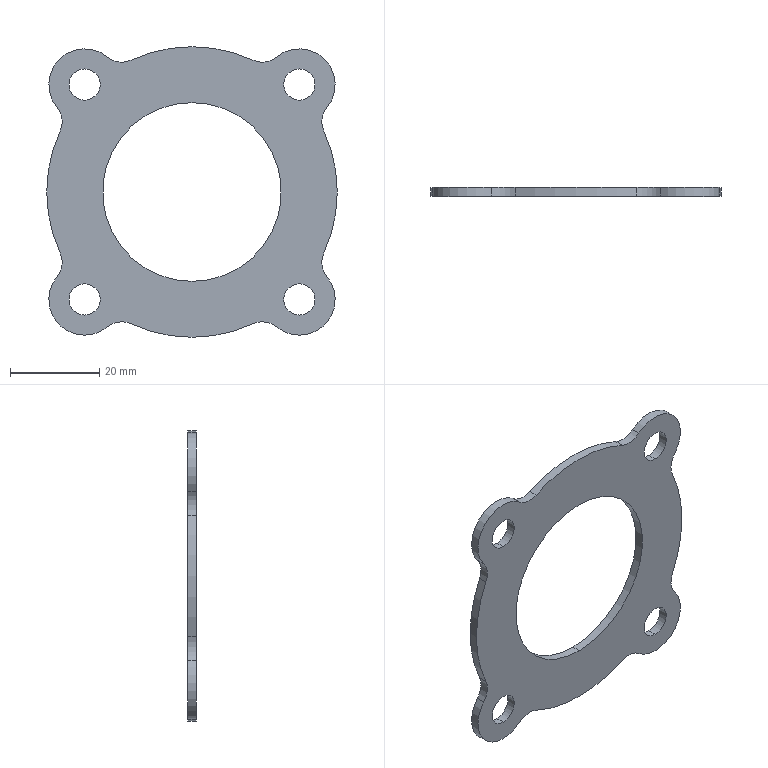Part | SolidWorks | features Fillet 2, Extrusion 1 | 1 solid | 33 faces | box 65 x 2 x 65 mm | volume 4890 mm3 | cylinder 31 | plane 2 | commonest cylinder face diameters 10 x10 7 x8 16 x6 65 x5 40 x2
STEP:
#1=CARTESIAN_POINT('',(-15.733,0.,-29.04));
#2=VERTEX_POINT('',#1);
#3=CARTESIAN_POINT('',(-13.635,0.,-29.501));
#4=VERTEX_POINT('',#3);
#5=CARTESIAN_POINT('',(-15.733,0.,-34.04));
#6=DIRECTION('',(0.,1.,0.));
#7=DIRECTION('',(0.,0.,1.));
#8=AXIS2_PLACEMENT_3D('',#5,#6,#7);
#9=CIRCLE('',#8,5.);
#10=EDGE_CURVE('',#2,#4,#9,.T.);
#11=ORIENTED_EDGE('',*,*,#10,.F.);
#12=CARTESIAN_POINT('',(-15.733,2.,-29.04));
#13=VERTEX_POINT('',#12);
#14=CARTESIAN_POINT('',(-15.733,2.,-29.04));
#15=DIRECTION('',(0.,1.,0.));
#16=VECTOR('',#15,1000.);
#17=LINE('',#14,#16);
#18=EDGE_CURVE('',#2,#13,#17,.T.);
#19=ORIENTED_EDGE('',*,*,#18,.T.);
#20=CARTESIAN_POINT('',(-13.635,2.,-29.501));
#21=VERTEX_POINT('',#20);
#22=CARTESIAN_POINT('',(-15.733,2.,-34.04));
#23=DIRECTION('',(0.,-1.,0.));
#24=DIRECTION('',(0.,0.,1.));
#25=AXIS2_PLACEMENT_3D('',#22,#23,#24);
#26=CIRCLE('',#25,5.);
#27=EDGE_CURVE('',#21,#13,#26,.T.);
#28=ORIENTED_EDGE('',*,*,#27,.F.);
#29=CARTESIAN_POINT('',(-13.635,2.,-29.501));
#30=DIRECTION('',(0.,1.,0.));
#31=VECTOR('',#30,1000.);
#32=LINE('',#29,#31);
#33=EDGE_CURVE('',#4,#21,#32,.T.);
#34=ORIENTED_EDGE('',*,*,#33,.F.);
#35=EDGE_LOOP('',(#11,#19,#28,#34));
#36=FACE_OUTER_BOUND('',#35,.T.);
#37=CARTESIAN_POINT('',(-15.733,2.,-34.04));
#38=DIRECTION('',(0.,1.,0.));
#39=DIRECTION('',(0.,0.,1.));
#40=AXIS2_PLACEMENT_3D('',#37,#38,#39);
#41=CYLINDRICAL_SURFACE('',#40,5.);
#42=ADVANCED_FACE('',(#36),#41,.F.);
#43=CARTESIAN_POINT('',(15.733,0.,-29.04));
#44=VERTEX_POINT('',#43);
#45=CARTESIAN_POINT('',(18.929,0.,-30.194));
#46=VERTEX_POINT('',#45);
#47=CARTESIAN_POINT('',(15.733,0.,-34.04));
#48=DIRECTION('',(0.,1.,0.));
#49=DIRECTION('',(0.,0.,1.));
#50=AXIS2_PLACEMENT_3D('',#47,#48,#49);
#51=CIRCLE('',#50,5.);
#52=EDGE_CURVE('',#44,#46,#51,.T.);
#53=ORIENTED_EDGE('',*,*,#52,.F.);
#54=CARTESIAN_POINT('',(15.733,2.,-29.04));
#55=VERTEX_POINT('',#54);
#56=CARTESIAN_POINT('',(15.733,2.,-29.04));
#57=DIRECTION('',(0.,1.,0.));
#58=VECTOR('',#57,1000.);
#59=LINE('',#56,#58);
#60=EDGE_CURVE('',#44,#55,#59,.T.);
#61=ORIENTED_EDGE('',*,*,#60,.T.);
#62=CARTESIAN_POINT('',(18.929,2.,-30.194));
#63=VERTEX_POINT('',#62);
#64=CARTESIAN_POINT('',(15.733,2.,-34.04));
#65=DIRECTION('',(0.,-1.,0.));
#66=DIRECTION('',(0.,0.,1.));
#67=AXIS2_PLACEMENT_3D('',#64,#65,#66);
#68=CIRCLE('',#67,5.);
#69=EDGE_CURVE('',#63,#55,#68,.T.);
#70=ORIENTED_EDGE('',*,*,#69,.F.);
#71=CARTESIAN_POINT('',(18.929,2.,-30.194));
#72=DIRECTION('',(0.,1.,0.));
#73=VECTOR('',#72,1000.);
#74=LINE('',#71,#73);
#75=EDGE_CURVE('',#46,#63,#74,.T.);
#76=ORIENTED_EDGE('',*,*,#75,.F.);
#77=EDGE_LOOP('',(#53,#61,#70,#76));
#78=FACE_OUTER_BOUND('',#77,.T.);
#79=CARTESIAN_POINT('',(15.733,2.,-34.04));
#80=DIRECTION('',(0.,1.,0.));
#81=DIRECTION('',(0.,0.,1.));
#82=AXIS2_PLACEMENT_3D('',#79,#80,#81);
#83=CYLINDRICAL_SURFACE('',#82,5.);
#84=ADVANCED_FACE('',(#78),#83,.F.);
#85=CARTESIAN_POINT('',(-24.042,2.,20.542));
#86=VERTEX_POINT('',#85);
#87=CARTESIAN_POINT('',(-24.042,2.,27.542));
#88=VERTEX_POINT('',#87);
#89=CARTESIAN_POINT('',(-24.042,2.,24.042));
#90=DIRECTION('',(0.,1.,0.));
#91=DIRECTION('',(0.,0.,1.));
#92=AXIS2_PLACEMENT_3D('',#89,#90,#91);
#93=CIRCLE('',#92,3.5);
#94=EDGE_CURVE('',#86,#88,#93,.T.);
#95=ORIENTED_EDGE('',*,*,#94,.T.);
#96=CARTESIAN_POINT('',(-24.042,0.,27.542));
#97=VERTEX_POINT('',#96);
#98=CARTESIAN_POINT('',(-24.042,2.,27.542));
#99=DIRECTION('',(0.,-1.,0.));
#100=VECTOR('',#99,1000.);
#101=LINE('',#98,#100);
#102=EDGE_CURVE('',#88,#97,#101,.T.);
#103=ORIENTED_EDGE('',*,*,#102,.T.);
#104=CARTESIAN_POINT('',(-24.042,0.,20.542));
#105=VERTEX_POINT('',#104);
#106=CARTESIAN_POINT('',(-24.042,0.,24.042));
#107=DIRECTION('',(0.,1.,0.));
#108=DIRECTION('',(0.,0.,1.));
#109=AXIS2_PLACEMENT_3D('',#106,#107,#108);
#110=CIRCLE('',#109,3.5);
#111=EDGE_CURVE('',#105,#97,#110,.T.);
#112=ORIENTED_EDGE('',*,*,#111,.F.);
#113=CARTESIAN_POINT('',(-24.042,2.,20.542));
#114=DIRECTION('',(0.,-1.,0.));
#115=VECTOR('',#114,1000.);
#116=LINE('',#113,#115);
#117=EDGE_CURVE('',#86,#105,#116,.T.);
#118=ORIENTED_EDGE('',*,*,#117,.F.);
#119=EDGE_LOOP('',(#95,#103,#112,#118));
#120=FACE_OUTER_BOUND('',#119,.T.);
#121=CARTESIAN_POINT('',(-24.042,2.,24.042));
#122=DIRECTION('',(0.,-1.,0.));
#123=DIRECTION('',(0.,0.,-1.));
#124=AXIS2_PLACEMENT_3D('',#121,#122,#123);
#125=CYLINDRICAL_SURFACE('',#124,3.5);
#126=ADVANCED_FACE('',(#120),#125,.F.);
#127=CARTESIAN_POINT('',(24.042,2.,20.542));
#128=VERTEX_POINT('',#127);
#129=CARTESIAN_POINT('',(24.042,2.,27.542));
#130=VERTEX_POINT('',#129);
#131=CARTESIAN_POINT('',(24.042,2.,24.042));
#132=DIRECTION('',(0.,1.,0.));
#133=DIRECTION('',(0.,0.,1.));
#134=AXIS2_PLACEMENT_3D('',#131,#132,#133);
#135=CIRCLE('',#134,3.5);
#136=EDGE_CURVE('',#128,#130,#135,.T.);
#137=ORIENTED_EDGE('',*,*,#136,.T.);
#138=CARTESIAN_POINT('',(24.042,0.,27.542));
#139=VERTEX_POINT('',#138);
#140=CARTESIAN_POINT('',(24.042,2.,27.542));
#141=DIRECTION('',(0.,-1.,0.));
#142=VECTOR('',#141,1000.);
#143=LINE('',#140,#142);
#144=EDGE_CURVE('',#130,#139,#143,.T.);
#145=ORIENTED_EDGE('',*,*,#144,.T.);
#146=CARTESIAN_POINT('',(24.042,0.,20.542));
#147=VERTEX_POINT('',#146);
#148=CARTESIAN_POINT('',(24.042,0.,24.042));
#149=DIRECTION('',(0.,1.,0.));
#150=DIRECTION('',(0.,0.,1.));
#151=AXIS2_PLACEMENT_3D('',#148,#149,#150);
#152=CIRCLE('',#151,3.5);
#153=EDGE_CURVE('',#147,#139,#152,.T.);
#154=ORIENTED_EDGE('',*,*,#153,.F.);
#155=CARTESIAN_POINT('',(24.042,2.,20.542));
#156=DIRECTION('',(0.,-1.,0.));
#157=VECTOR('',#156,1000.);
#158=LINE('',#155,#157);
#159=EDGE_CURVE('',#128,#147,#158,.T.);
#160=ORIENTED_EDGE('',*,*,#159,.F.);
#161=EDGE_LOOP('',(#137,#145,#154,#160));
#162=FACE_OUTER_BOUND('',#161,.T.);
#163=CARTESIAN_POINT('',(24.042,2.,24.042));
#164=DIRECTION('',(0.,-1.,0.));
#165=DIRECTION('',(0.,0.,-1.));
#166=AXIS2_PLACEMENT_3D('',#163,#164,#165);
#167=CYLINDRICAL_SURFACE('',#166,3.5);
#168=ADVANCED_FACE('',(#162),#167,.F.);
#169=CARTESIAN_POINT('',(24.042,2.,-27.542));
#170=VERTEX_POINT('',#169);
#171=CARTESIAN_POINT('',(24.042,2.,-20.542));
#172=VERTEX_POINT('',#171);
#173=CARTESIAN_POINT('',(24.042,2.,-24.042));
#174=DIRECTION('',(0.,1.,0.));
#175=DIRECTION('',(0.,0.,1.));
#176=AXIS2_PLACEMENT_3D('',#173,#174,#175);
#177=CIRCLE('',#176,3.5);
#178=EDGE_CURVE('',#170,#172,#177,.T.);
#179=ORIENTED_EDGE('',*,*,#178,.T.);
#180=CARTESIAN_POINT('',(24.042,0.,-20.542));
#181=VERTEX_POINT('',#180);
#182=CARTESIAN_POINT('',(24.042,2.,-20.542));
#183=DIRECTION('',(0.,-1.,0.));
#184=VECTOR('',#183,1000.);
#185=LINE('',#182,#184);
#186=EDGE_CURVE('',#172,#181,#185,.T.);
#187=ORIENTED_EDGE('',*,*,#186,.T.);
#188=CARTESIAN_POINT('',(24.042,0.,-27.542));
#189=VERTEX_POINT('',#188);
#190=CARTESIAN_POINT('',(24.042,0.,-24.042));
#191=DIRECTION('',(0.,1.,0.));
#192=DIRECTION('',(0.,0.,1.));
#193=AXIS2_PLACEMENT_3D('',#190,#191,#192);
#194=CIRCLE('',#193,3.5);
#195=EDGE_CURVE('',#189,#181,#194,.T.);
#196=ORIENTED_EDGE('',*,*,#195,.F.);
#197=CARTESIAN_POINT('',(24.042,2.,-27.542));
#198=DIRECTION('',(0.,-1.,0.));
#199=VECTOR('',#198,1000.);
#200=LINE('',#197,#199);
#201=EDGE_CURVE('',#170,#189,#200,.T.);
#202=ORIENTED_EDGE('',*,*,#201,.F.);
#203=EDGE_LOOP('',(#179,#187,#196,#202));
#204=FACE_OUTER_BOUND('',#203,.T.);
#205=CARTESIAN_POINT('',(24.042,2.,-24.042));
#206=DIRECTION('',(0.,-1.,0.));
#207=DIRECTION('',(0.,0.,-1.));
#208=AXIS2_PLACEMENT_3D('',#205,#206,#207);
#209=CYLINDRICAL_SURFACE('',#208,3.5);
#210=ADVANCED_FACE('',(#204),#209,.F.);
#211=CARTESIAN_POINT('',(-24.042,2.,-27.542));
#212=VERTEX_POINT('',#211);
#213=CARTESIAN_POINT('',(-24.042,2.,-20.542));
#214=VERTEX_POINT('',#213);
#215=CARTESIAN_POINT('',(-24.042,2.,-24.042));
#216=DIRECTION('',(0.,1.,0.));
#217=DIRECTION('',(0.,0.,1.));
#218=AXIS2_PLACEMENT_3D('',#215,#216,#217);
#219=CIRCLE('',#218,3.5);
#220=EDGE_CURVE('',#212,#214,#219,.T.);
#221=ORIENTED_EDGE('',*,*,#220,.T.);
#222=CARTESIAN_POINT('',(-24.042,0.,-20.542));
#223=VERTEX_POINT('',#222);
#224=CARTESIAN_POINT('',(-24.042,2.,-20.542));
#225=DIRECTION('',(0.,-1.,0.));
#226=VECTOR('',#225,1000.);
#227=LINE('',#224,#226);
#228=EDGE_CURVE('',#214,#223,#227,.T.);
#229=ORIENTED_EDGE('',*,*,#228,.T.);
#230=CARTESIAN_POINT('',(-24.042,0.,-27.542));
#231=VERTEX_POINT('',#230);
#232=CARTESIAN_POINT('',(-24.042,0.,-24.042));
#233=DIRECTION('',(0.,1.,0.));
#234=DIRECTION('',(0.,0.,1.));
#235=AXIS2_PLACEMENT_3D('',#232,#233,#234);
#236=CIRCLE('',#235,3.5);
#237=EDGE_CURVE('',#231,#223,#236,.T.);
#238=ORIENTED_EDGE('',*,*,#237,.F.);
#239=CARTESIAN_POINT('',(-24.042,2.,-27.542));
#240=DIRECTION('',(0.,-1.,0.));
#241=VECTOR('',#240,1000.);
#242=LINE('',#239,#241);
#243=EDGE_CURVE('',#212,#231,#242,.T.);
#244=ORIENTED_EDGE('',*,*,#243,.F.);
#245=EDGE_LOOP('',(#221,#229,#238,#244));
#246=FACE_OUTER_BOUND('',#245,.T.);
#247=CARTESIAN_POINT('',(-24.042,2.,-24.042));
#248=DIRECTION('',(0.,-1.,0.));
#249=DIRECTION('',(0.,0.,-1.));
#250=AXIS2_PLACEMENT_3D('',#247,#248,#249);
#251=CYLINDRICAL_SURFACE('',#250,3.5);
#252=ADVANCED_FACE('',(#246),#251,.F.);
#253=CARTESIAN_POINT('',(0.,2.,-20.));
#254=VERTEX_POINT('',#253);
#255=CARTESIAN_POINT('',(0.,2.,20.));
#256=VERTEX_POINT('',#255);
#257=CARTESIAN_POINT('',(0.,2.,0.));
#258=DIRECTION('',(0.,1.,0.));
#259=DIRECTION('',(0.,0.,1.));
#260=AXIS2_PLACEMENT_3D('',#257,#258,#259);
#261=CIRCLE('',#260,20.);
#262=EDGE_CURVE('',#254,#256,#261,.T.);
#263=ORIENTED_EDGE('',*,*,#262,.T.);
#264=CARTESIAN_POINT('',(0.,0.,20.));
#265=VERTEX_POINT('',#264);
#266=CARTESIAN_POINT('',(0.,2.,20.));
#267=DIRECTION('',(0.,-1.,0.));
#268=VECTOR('',#267,1000.);
#269=LINE('',#266,#268);
#270=EDGE_CURVE('',#256,#265,#269,.T.);
#271=ORIENTED_EDGE('',*,*,#270,.T.);
#272=CARTESIAN_POINT('',(0.,0.,-20.));
#273=VERTEX_POINT('',#272);
#274=CARTESIAN_POINT('',(0.,0.,0.));
#275=DIRECTION('',(0.,1.,0.));
#276=DIRECTION('',(0.,0.,1.));
#277=AXIS2_PLACEMENT_3D('',#274,#275,#276);
#278=CIRCLE('',#277,20.);
#279=EDGE_CURVE('',#273,#265,#278,.T.);
#280=ORIENTED_EDGE('',*,*,#279,.F.);
#281=CARTESIAN_POINT('',(0.,2.,-20.));
#282=DIRECTION('',(0.,-1.,0.));
#283=VECTOR('',#282,1000.);
#284=LINE('',#281,#283);
#285=EDGE_CURVE('',#254,#273,#284,.T.);
#286=ORIENTED_EDGE('',*,*,#285,.F.);
#287=EDGE_LOOP('',(#263,#271,#280,#286));
#288=FACE_OUTER_BOUND('',#287,.T.);
#289=CARTESIAN_POINT('',(0.,2.,0.));
#290=DIRECTION('',(0.,-1.,0.));
#291=DIRECTION('',(0.,0.,-1.));
#292=AXIS2_PLACEMENT_3D('',#289,#290,#291);
#293=CYLINDRICAL_SURFACE('',#292,20.);
#294=ADVANCED_FACE('',(#288),#293,.F.);
#295=CARTESIAN_POINT('',(24.042,2.,-32.042));
#296=VERTEX_POINT('',#295);
#297=CARTESIAN_POINT('',(24.042,2.,-24.042));
#298=DIRECTION('',(0.,1.,0.));
#299=DIRECTION('',(0.,0.,1.));
#300=AXIS2_PLACEMENT_3D('',#297,#298,#299);
#301=CIRCLE('',#300,8.);
#302=EDGE_CURVE('',#296,#63,#301,.T.);
#303=ORIENTED_EDGE('',*,*,#302,.F.);
#304=CARTESIAN_POINT('',(24.042,0.,-32.042));
#305=VERTEX_POINT('',#304);
#306=CARTESIAN_POINT('',(24.042,2.,-32.042));
#307=DIRECTION('',(0.,-1.,0.));
#308=VECTOR('',#307,1000.);
#309=LINE('',#306,#308);
#310=EDGE_CURVE('',#296,#305,#309,.T.);
#311=ORIENTED_EDGE('',*,*,#310,.T.);
#312=CARTESIAN_POINT('',(24.042,0.,-24.042));
#313=DIRECTION('',(0.,1.,0.));
#314=DIRECTION('',(0.,0.,1.));
#315=AXIS2_PLACEMENT_3D('',#312,#313,#314);
#316=CIRCLE('',#315,8.);
#317=EDGE_CURVE('',#305,#46,#316,.T.);
#318=ORIENTED_EDGE('',*,*,#317,.T.);
#319=ORIENTED_EDGE('',*,*,#75,.T.);
#320=EDGE_LOOP('',(#303,#311,#318,#319));
#321=FACE_OUTER_BOUND('',#320,.T.);
#322=CARTESIAN_POINT('',(24.042,2.,-24.042));
#323=DIRECTION('',(0.,-1.,0.));
#324=DIRECTION('',(0.,0.,-1.));
#325=AXIS2_PLACEMENT_3D('',#322,#323,#324);
#326=CYLINDRICAL_SURFACE('',#325,8.);
#327=ADVANCED_FACE('',(#321),#326,.T.);
#328=CARTESIAN_POINT('',(-24.042,2.,-32.042));
#329=VERTEX_POINT('',#328);
#330=CARTESIAN_POINT('',(-30.194,2.,-18.929));
#331=VERTEX_POINT('',#330);
#332=CARTESIAN_POINT('',(-24.042,2.,-24.042));
#333=DIRECTION('',(0.,1.,0.));
#334=DIRECTION('',(0.,0.,1.));
#335=AXIS2_PLACEMENT_3D('',#332,#333,#334);
#336=CIRCLE('',#335,8.);
#337=EDGE_CURVE('',#329,#331,#336,.T.);
#338=ORIENTED_EDGE('',*,*,#337,.F.);
#339=CARTESIAN_POINT('',(-24.042,0.,-32.042));
#340=VERTEX_POINT('',#339);
#341=CARTESIAN_POINT('',(-24.042,2.,-32.042));
#342=DIRECTION('',(0.,-1.,0.));
#343=VECTOR('',#342,1000.);
#344=LINE('',#341,#343);
#345=EDGE_CURVE('',#329,#340,#344,.T.);
#346=ORIENTED_EDGE('',*,*,#345,.T.);
#347=CARTESIAN_POINT('',(-30.194,0.,-18.929));
#348=VERTEX_POINT('',#347);
#349=CARTESIAN_POINT('',(-24.042,0.,-24.042));
#350=DIRECTION('',(0.,1.,0.));
#351=DIRECTION('',(0.,0.,1.));
#352=AXIS2_PLACEMENT_3D('',#349,#350,#351);
#353=CIRCLE('',#352,8.);
#354=EDGE_CURVE('',#340,#348,#353,.T.);
#355=ORIENTED_EDGE('',*,*,#354,.T.);
#356=CARTESIAN_POINT('',(-30.194,2.,-18.929));
#357=DIRECTION('',(0.,1.,0.));
#358=VECTOR('',#357,1000.);
#359=LINE('',#356,#358);
#360=EDGE_CURVE('',#348,#331,#359,.T.);
#361=ORIENTED_EDGE('',*,*,#360,.T.);
#362=EDGE_LOOP('',(#338,#346,#355,#361));
#363=FACE_OUTER_BOUND('',#362,.T.);
#364=CARTESIAN_POINT('',(-24.042,2.,-24.042));
#365=DIRECTION('',(0.,-1.,0.));
#366=DIRECTION('',(0.,0.,-1.));
#367=AXIS2_PLACEMENT_3D('',#364,#365,#366);
#368=CYLINDRICAL_SURFACE('',#367,8.);
#369=ADVANCED_FACE('',(#363),#368,.T.);
#370=CARTESIAN_POINT('',(0.,2.,-32.5));
#371=VERTEX_POINT('',#370);
#372=CARTESIAN_POINT('',(0.,2.,0.));
#373=DIRECTION('',(0.,1.,0.));
#374=DIRECTION('',(0.,0.,1.));
#375=AXIS2_PLACEMENT_3D('',#372,#373,#374);
#376=CIRCLE('',#375,32.5);
#377=EDGE_CURVE('',#371,#21,#376,.T.);
#378=ORIENTED_EDGE('',*,*,#377,.F.);
#379=CARTESIAN_POINT('',(0.,0.,-32.5));
#380=VERTEX_POINT('',#379);
#381=CARTESIAN_POINT('',(0.,2.,-32.5));
#382=DIRECTION('',(0.,-1.,0.));
#383=VECTOR('',#382,1000.);
#384=LINE('',#381,#383);
#385=EDGE_CURVE('',#371,#380,#384,.T.);
#386=ORIENTED_EDGE('',*,*,#385,.T.);
#387=CARTESIAN_POINT('',(0.,0.,0.));
#388=DIRECTION('',(0.,1.,0.));
#389=DIRECTION('',(0.,0.,1.));
#390=AXIS2_PLACEMENT_3D('',#387,#388,#389);
#391=CIRCLE('',#390,32.5);
#392=EDGE_CURVE('',#380,#4,#391,.T.);
#393=ORIENTED_EDGE('',*,*,#392,.T.);
#394=ORIENTED_EDGE('',*,*,#33,.T.);
#395=EDGE_LOOP('',(#378,#386,#393,#394));
#396=FACE_OUTER_BOUND('',#395,.T.);
#397=CARTESIAN_POINT('',(0.,2.,0.));
#398=DIRECTION('',(0.,-1.,0.));
#399=DIRECTION('',(0.,0.,-1.));
#400=AXIS2_PLACEMENT_3D('',#397,#398,#399);
#401=CYLINDRICAL_SURFACE('',#400,32.5);
#402=ADVANCED_FACE('',(#396),#401,.T.);
#403=ORIENTED_EDGE('',*,*,#136,.F.);
#404=CARTESIAN_POINT('',(24.042,2.,24.042));
#405=DIRECTION('',(0.,1.,0.));
#406=DIRECTION('',(0.,0.,1.));
#407=AXIS2_PLACEMENT_3D('',#404,#405,#406);
#408=CIRCLE('',#407,3.5);
#409=EDGE_CURVE('',#130,#128,#408,.T.);
#410=ORIENTED_EDGE('',*,*,#409,.F.);
#411=EDGE_LOOP('',(#403,#410));
#412=FACE_BOUND('',#411,.T.);
#413=ORIENTED_EDGE('',*,*,#220,.F.);
#414=CARTESIAN_POINT('',(-24.042,2.,-24.042));
#415=DIRECTION('',(0.,1.,0.));
#416=DIRECTION('',(0.,0.,1.));
#417=AXIS2_PLACEMENT_3D('',#414,#415,#416);
#418=CIRCLE('',#417,3.5);
#419=EDGE_CURVE('',#214,#212,#418,.T.);
#420=ORIENTED_EDGE('',*,*,#419,.F.);
#421=EDGE_LOOP('',(#413,#420));
#422=FACE_BOUND('',#421,.T.);
#423=CARTESIAN_POINT('',(30.194,2.,-18.929));
#424=VERTEX_POINT('',#423);
#425=CARTESIAN_POINT('',(24.042,2.,-24.042));
#426=DIRECTION('',(0.,1.,0.));
#427=DIRECTION('',(0.,0.,1.));
#428=AXIS2_PLACEMENT_3D('',#425,#426,#427);
#429=CIRCLE('',#428,8.);
#430=EDGE_CURVE('',#424,#296,#429,.T.);
#431=ORIENTED_EDGE('',*,*,#430,.T.);
#432=ORIENTED_EDGE('',*,*,#302,.T.);
#433=ORIENTED_EDGE('',*,*,#69,.T.);
#434=CARTESIAN_POINT('',(13.635,2.,-29.501));
#435=VERTEX_POINT('',#434);
#436=CARTESIAN_POINT('',(15.733,2.,-34.04));
#437=DIRECTION('',(0.,-1.,0.));
#438=DIRECTION('',(0.,0.,1.));
#439=AXIS2_PLACEMENT_3D('',#436,#437,#438);
#440=CIRCLE('',#439,5.);
#441=EDGE_CURVE('',#55,#435,#440,.T.);
#442=ORIENTED_EDGE('',*,*,#441,.T.);
#443=CARTESIAN_POINT('',(0.,2.,0.));
#444=DIRECTION('',(0.,1.,0.));
#445=DIRECTION('',(0.,0.,1.));
#446=AXIS2_PLACEMENT_3D('',#443,#444,#445);
#447=CIRCLE('',#446,32.5);
#448=EDGE_CURVE('',#435,#371,#447,.T.);
#449=ORIENTED_EDGE('',*,*,#448,.T.);
#450=ORIENTED_EDGE('',*,*,#377,.T.);
#451=ORIENTED_EDGE('',*,*,#27,.T.);
#452=CARTESIAN_POINT('',(-18.929,2.,-30.194));
#453=VERTEX_POINT('',#452);
#454=CARTESIAN_POINT('',(-15.733,2.,-34.04));
#455=DIRECTION('',(0.,-1.,0.));
#456=DIRECTION('',(0.,0.,1.));
#457=AXIS2_PLACEMENT_3D('',#454,#455,#456);
#458=CIRCLE('',#457,5.);
#459=EDGE_CURVE('',#13,#453,#458,.T.);
#460=ORIENTED_EDGE('',*,*,#459,.T.);
#461=CARTESIAN_POINT('',(-24.042,2.,-24.042));
#462=DIRECTION('',(0.,1.,0.));
#463=DIRECTION('',(0.,0.,1.));
#464=AXIS2_PLACEMENT_3D('',#461,#462,#463);
#465=CIRCLE('',#464,8.);
#466=EDGE_CURVE('',#453,#329,#465,.T.);
#467=ORIENTED_EDGE('',*,*,#466,.T.);
#468=ORIENTED_EDGE('',*,*,#337,.T.);
#469=CARTESIAN_POINT('',(-29.501,2.,-13.635));
#470=VERTEX_POINT('',#469);
#471=CARTESIAN_POINT('',(-34.04,2.,-15.733));
#472=DIRECTION('',(0.,-1.,0.));
#473=DIRECTION('',(0.,0.,1.));
#474=AXIS2_PLACEMENT_3D('',#471,#472,#473);
#475=CIRCLE('',#474,5.);
#476=EDGE_CURVE('',#331,#470,#475,.T.);
#477=ORIENTED_EDGE('',*,*,#476,.T.);
#478=CARTESIAN_POINT('',(-29.501,2.,13.635));
#479=VERTEX_POINT('',#478);
#480=CARTESIAN_POINT('',(0.,2.,0.));
#481=DIRECTION('',(0.,1.,0.));
#482=DIRECTION('',(0.,0.,1.));
#483=AXIS2_PLACEMENT_3D('',#480,#481,#482);
#484=CIRCLE('',#483,32.5);
#485=EDGE_CURVE('',#470,#479,#484,.T.);
#486=ORIENTED_EDGE('',*,*,#485,.T.);
#487=CARTESIAN_POINT('',(-30.194,2.,18.929));
#488=VERTEX_POINT('',#487);
#489=CARTESIAN_POINT('',(-34.04,2.,15.733));
#490=DIRECTION('',(0.,-1.,0.));
#491=DIRECTION('',(0.,0.,1.));
#492=AXIS2_PLACEMENT_3D('',#489,#490,#491);
#493=CIRCLE('',#492,5.);
#494=EDGE_CURVE('',#479,#488,#493,.T.);
#495=ORIENTED_EDGE('',*,*,#494,.T.);
#496=CARTESIAN_POINT('',(-18.929,2.,30.194));
#497=VERTEX_POINT('',#496);
#498=CARTESIAN_POINT('',(-24.042,2.,24.042));
#499=DIRECTION('',(0.,1.,0.));
#500=DIRECTION('',(0.,0.,1.));
#501=AXIS2_PLACEMENT_3D('',#498,#499,#500);
#502=CIRCLE('',#501,8.);
#503=EDGE_CURVE('',#488,#497,#502,.T.);
#504=ORIENTED_EDGE('',*,*,#503,.T.);
#505=CARTESIAN_POINT('',(-13.635,2.,29.501));
#506=VERTEX_POINT('',#505);
#507=CARTESIAN_POINT('',(-15.733,2.,34.04));
#508=DIRECTION('',(0.,-1.,0.));
#509=DIRECTION('',(0.,0.,1.));
#510=AXIS2_PLACEMENT_3D('',#507,#508,#509);
#511=CIRCLE('',#510,5.);
#512=EDGE_CURVE('',#497,#506,#511,.T.);
#513=ORIENTED_EDGE('',*,*,#512,.T.);
#514=CARTESIAN_POINT('',(13.635,2.,29.501));
#515=VERTEX_POINT('',#514);
#516=CARTESIAN_POINT('',(0.,2.,0.));
#517=DIRECTION('',(0.,1.,0.));
#518=DIRECTION('',(0.,0.,1.));
#519=AXIS2_PLACEMENT_3D('',#516,#517,#518);
#520=CIRCLE('',#519,32.5);
#521=EDGE_CURVE('',#506,#515,#520,.T.);
#522=ORIENTED_EDGE('',*,*,#521,.T.);
#523=CARTESIAN_POINT('',(18.929,2.,30.194));
#524=VERTEX_POINT('',#523);
#525=CARTESIAN_POINT('',(15.733,2.,34.04));
#526=DIRECTION('',(0.,-1.,0.));
#527=DIRECTION('',(0.,0.,1.));
#528=AXIS2_PLACEMENT_3D('',#525,#526,#527);
#529=CIRCLE('',#528,5.);
#530=EDGE_CURVE('',#515,#524,#529,.T.);
#531=ORIENTED_EDGE('',*,*,#530,.T.);
#532=CARTESIAN_POINT('',(30.194,2.,18.929));
#533=VERTEX_POINT('',#532);
#534=CARTESIAN_POINT('',(24.042,2.,24.042));
#535=DIRECTION('',(0.,1.,0.));
#536=DIRECTION('',(0.,0.,1.));
#537=AXIS2_PLACEMENT_3D('',#534,#535,#536);
#538=CIRCLE('',#537,8.);
#539=EDGE_CURVE('',#524,#533,#538,.T.);
#540=ORIENTED_EDGE('',*,*,#539,.T.);
#541=CARTESIAN_POINT('',(29.501,2.,13.635));
#542=VERTEX_POINT('',#541);
#543=CARTESIAN_POINT('',(34.04,2.,15.733));
#544=DIRECTION('',(0.,-1.,0.));
#545=DIRECTION('',(0.,0.,1.));
#546=AXIS2_PLACEMENT_3D('',#543,#544,#545);
#547=CIRCLE('',#546,5.);
#548=EDGE_CURVE('',#533,#542,#547,.T.);
#549=ORIENTED_EDGE('',*,*,#548,.T.);
#550=CARTESIAN_POINT('',(29.501,2.,-13.635));
#551=VERTEX_POINT('',#550);
#552=CARTESIAN_POINT('',(0.,2.,0.));
#553=DIRECTION('',(0.,1.,0.));
#554=DIRECTION('',(0.,0.,1.));
#555=AXIS2_PLACEMENT_3D('',#552,#553,#554);
#556=CIRCLE('',#555,32.5);
#557=EDGE_CURVE('',#542,#551,#556,.T.);
#558=ORIENTED_EDGE('',*,*,#557,.T.);
#559=CARTESIAN_POINT('',(34.04,2.,-15.733));
#560=DIRECTION('',(0.,-1.,0.));
#561=DIRECTION('',(0.,0.,1.));
#562=AXIS2_PLACEMENT_3D('',#559,#560,#561);
#563=CIRCLE('',#562,5.);
#564=EDGE_CURVE('',#551,#424,#563,.T.);
#565=ORIENTED_EDGE('',*,*,#564,.T.);
#566=EDGE_LOOP('',(#431,#432,#433,#442,#449,#450,#451,#460,#467,#468,#477,#486,#495,#504,#513,#522,#531,#540,#549,#558,#565));
#567=FACE_OUTER_BOUND('',#566,.T.);
#568=ORIENTED_EDGE('',*,*,#262,.F.);
#569=CARTESIAN_POINT('',(0.,2.,0.));
#570=DIRECTION('',(0.,1.,0.));
#571=DIRECTION('',(0.,0.,1.));
#572=AXIS2_PLACEMENT_3D('',#569,#570,#571);
#573=CIRCLE('',#572,20.);
#574=EDGE_CURVE('',#256,#254,#573,.T.);
#575=ORIENTED_EDGE('',*,*,#574,.F.);
#576=EDGE_LOOP('',(#568,#575));
#577=FACE_BOUND('',#576,.T.);
#578=ORIENTED_EDGE('',*,*,#178,.F.);
#579=CARTESIAN_POINT('',(24.042,2.,-24.042));
#580=DIRECTION('',(0.,1.,0.));
#581=DIRECTION('',(0.,0.,1.));
#582=AXIS2_PLACEMENT_3D('',#579,#580,#581);
#583=CIRCLE('',#582,3.5);
#584=EDGE_CURVE('',#172,#170,#583,.T.);
#585=ORIENTED_EDGE('',*,*,#584,.F.);
#586=EDGE_LOOP('',(#578,#585));
#587=FACE_BOUND('',#586,.T.);
#588=ORIENTED_EDGE('',*,*,#94,.F.);
#589=CARTESIAN_POINT('',(-24.042,2.,24.042));
#590=DIRECTION('',(0.,1.,0.));
#591=DIRECTION('',(0.,0.,1.));
#592=AXIS2_PLACEMENT_3D('',#589,#590,#591);
#593=CIRCLE('',#592,3.5);
#594=EDGE_CURVE('',#88,#86,#593,.T.);
#595=ORIENTED_EDGE('',*,*,#594,.F.);
#596=EDGE_LOOP('',(#588,#595));
#597=FACE_BOUND('',#596,.T.);
#598=CARTESIAN_POINT('',(-12.021,2.,-12.021));
#599=DIRECTION('',(0.,1.,0.));
#600=DIRECTION('',(0.,0.,1.));
#601=AXIS2_PLACEMENT_3D('',#598,#599,#600);
#602=PLANE('',#601);
#603=ADVANCED_FACE('',(#412,#422,#567,#577,#587,#597),#602,.T.);
#604=CARTESIAN_POINT('',(13.635,0.,-29.501));
#605=VERTEX_POINT('',#604);
#606=CARTESIAN_POINT('',(0.,0.,0.));
#607=DIRECTION('',(0.,1.,0.));
#608=DIRECTION('',(0.,0.,1.));
#609=AXIS2_PLACEMENT_3D('',#606,#607,#608);
#610=CIRCLE('',#609,32.5);
#611=EDGE_CURVE('',#605,#380,#610,.T.);
#612=ORIENTED_EDGE('',*,*,#611,.F.);
#613=CARTESIAN_POINT('',(15.733,0.,-34.04));
#614=DIRECTION('',(0.,1.,0.));
#615=DIRECTION('',(0.,0.,1.));
#616=AXIS2_PLACEMENT_3D('',#613,#614,#615);
#617=CIRCLE('',#616,5.);
#618=EDGE_CURVE('',#605,#44,#617,.T.);
#619=ORIENTED_EDGE('',*,*,#618,.T.);
#620=ORIENTED_EDGE('',*,*,#52,.T.);
#621=ORIENTED_EDGE('',*,*,#317,.F.);
#622=CARTESIAN_POINT('',(30.194,0.,-18.929));
#623=VERTEX_POINT('',#622);
#624=CARTESIAN_POINT('',(24.042,0.,-24.042));
#625=DIRECTION('',(0.,1.,0.));
#626=DIRECTION('',(0.,0.,1.));
#627=AXIS2_PLACEMENT_3D('',#624,#625,#626);
#628=CIRCLE('',#627,8.);
#629=EDGE_CURVE('',#623,#305,#628,.T.);
#630=ORIENTED_EDGE('',*,*,#629,.F.);
#631=CARTESIAN_POINT('',(29.501,0.,-13.635));
#632=VERTEX_POINT('',#631);
#633=CARTESIAN_POINT('',(34.04,0.,-15.733));
#634=DIRECTION('',(0.,1.,0.));
#635=DIRECTION('',(0.,0.,1.));
#636=AXIS2_PLACEMENT_3D('',#633,#634,#635);
#637=CIRCLE('',#636,5.);
#638=EDGE_CURVE('',#623,#632,#637,.T.);
#639=ORIENTED_EDGE('',*,*,#638,.T.);
#640=CARTESIAN_POINT('',(29.501,0.,13.635));
#641=VERTEX_POINT('',#640);
#642=CARTESIAN_POINT('',(0.,0.,0.));
#643=DIRECTION('',(0.,1.,0.));
#644=DIRECTION('',(0.,0.,1.));
#645=AXIS2_PLACEMENT_3D('',#642,#643,#644);
#646=CIRCLE('',#645,32.5);
#647=EDGE_CURVE('',#641,#632,#646,.T.);
#648=ORIENTED_EDGE('',*,*,#647,.F.);
#649=CARTESIAN_POINT('',(30.194,0.,18.929));
#650=VERTEX_POINT('',#649);
#651=CARTESIAN_POINT('',(34.04,0.,15.733));
#652=DIRECTION('',(0.,1.,0.));
#653=DIRECTION('',(0.,0.,1.));
#654=AXIS2_PLACEMENT_3D('',#651,#652,#653);
#655=CIRCLE('',#654,5.);
#656=EDGE_CURVE('',#641,#650,#655,.T.);
#657=ORIENTED_EDGE('',*,*,#656,.T.);
#658=CARTESIAN_POINT('',(18.929,0.,30.194));
#659=VERTEX_POINT('',#658);
#660=CARTESIAN_POINT('',(24.042,0.,24.042));
#661=DIRECTION('',(0.,1.,0.));
#662=DIRECTION('',(0.,0.,1.));
#663=AXIS2_PLACEMENT_3D('',#660,#661,#662);
#664=CIRCLE('',#663,8.);
#665=EDGE_CURVE('',#659,#650,#664,.T.);
#666=ORIENTED_EDGE('',*,*,#665,.F.);
#667=CARTESIAN_POINT('',(13.635,0.,29.501));
#668=VERTEX_POINT('',#667);
#669=CARTESIAN_POINT('',(15.733,0.,34.04));
#670=DIRECTION('',(0.,1.,0.));
#671=DIRECTION('',(0.,0.,1.));
#672=AXIS2_PLACEMENT_3D('',#669,#670,#671);
#673=CIRCLE('',#672,5.);
#674=EDGE_CURVE('',#659,#668,#673,.T.);
#675=ORIENTED_EDGE('',*,*,#674,.T.);
#676=CARTESIAN_POINT('',(-13.635,0.,29.501));
#677=VERTEX_POINT('',#676);
#678=CARTESIAN_POINT('',(0.,0.,0.));
#679=DIRECTION('',(0.,1.,0.));
#680=DIRECTION('',(0.,0.,1.));
#681=AXIS2_PLACEMENT_3D('',#678,#679,#680);
#682=CIRCLE('',#681,32.5);
#683=EDGE_CURVE('',#677,#668,#682,.T.);
#684=ORIENTED_EDGE('',*,*,#683,.F.);
#685=CARTESIAN_POINT('',(-18.929,0.,30.194));
#686=VERTEX_POINT('',#685);
#687=CARTESIAN_POINT('',(-15.733,0.,34.04));
#688=DIRECTION('',(0.,1.,0.));
#689=DIRECTION('',(0.,0.,1.));
#690=AXIS2_PLACEMENT_3D('',#687,#688,#689);
#691=CIRCLE('',#690,5.);
#692=EDGE_CURVE('',#677,#686,#691,.T.);
#693=ORIENTED_EDGE('',*,*,#692,.T.);
#694=CARTESIAN_POINT('',(-30.194,0.,18.929));
#695=VERTEX_POINT('',#694);
#696=CARTESIAN_POINT('',(-24.042,0.,24.042));
#697=DIRECTION('',(0.,1.,0.));
#698=DIRECTION('',(0.,0.,1.));
#699=AXIS2_PLACEMENT_3D('',#696,#697,#698);
#700=CIRCLE('',#699,8.);
#701=EDGE_CURVE('',#695,#686,#700,.T.);
#702=ORIENTED_EDGE('',*,*,#701,.F.);
#703=CARTESIAN_POINT('',(-29.501,0.,13.635));
#704=VERTEX_POINT('',#703);
#705=CARTESIAN_POINT('',(-34.04,0.,15.733));
#706=DIRECTION('',(0.,1.,0.));
#707=DIRECTION('',(0.,0.,1.));
#708=AXIS2_PLACEMENT_3D('',#705,#706,#707);
#709=CIRCLE('',#708,5.);
#710=EDGE_CURVE('',#695,#704,#709,.T.);
#711=ORIENTED_EDGE('',*,*,#710,.T.);
#712=CARTESIAN_POINT('',(-29.501,0.,-13.635));
#713=VERTEX_POINT('',#712);
#714=CARTESIAN_POINT('',(0.,0.,0.));
#715=DIRECTION('',(0.,1.,0.));
#716=DIRECTION('',(0.,0.,1.));
#717=AXIS2_PLACEMENT_3D('',#714,#715,#716);
#718=CIRCLE('',#717,32.5);
#719=EDGE_CURVE('',#713,#704,#718,.T.);
#720=ORIENTED_EDGE('',*,*,#719,.F.);
#721=CARTESIAN_POINT('',(-34.04,0.,-15.733));
#722=DIRECTION('',(0.,1.,0.));
#723=DIRECTION('',(0.,0.,1.));
#724=AXIS2_PLACEMENT_3D('',#721,#722,#723);
#725=CIRCLE('',#724,5.);
#726=EDGE_CURVE('',#713,#348,#725,.T.);
#727=ORIENTED_EDGE('',*,*,#726,.T.);
#728=ORIENTED_EDGE('',*,*,#354,.F.);
#729=CARTESIAN_POINT('',(-18.929,0.,-30.194));
#730=VERTEX_POINT('',#729);
#731=CARTESIAN_POINT('',(-24.042,0.,-24.042));
#732=DIRECTION('',(0.,1.,0.));
#733=DIRECTION('',(0.,0.,1.));
#734=AXIS2_PLACEMENT_3D('',#731,#732,#733);
#735=CIRCLE('',#734,8.);
#736=EDGE_CURVE('',#730,#340,#735,.T.);
#737=ORIENTED_EDGE('',*,*,#736,.F.);
#738=CARTESIAN_POINT('',(-15.733,0.,-34.04));
#739=DIRECTION('',(0.,1.,0.));
#740=DIRECTION('',(0.,0.,1.));
#741=AXIS2_PLACEMENT_3D('',#738,#739,#740);
#742=CIRCLE('',#741,5.);
#743=EDGE_CURVE('',#730,#2,#742,.T.);
#744=ORIENTED_EDGE('',*,*,#743,.T.);
#745=ORIENTED_EDGE('',*,*,#10,.T.);
#746=ORIENTED_EDGE('',*,*,#392,.F.);
#747=EDGE_LOOP('',(#612,#619,#620,#621,#630,#639,#648,#657,#666,#675,#684,#693,#702,#711,#720,#727,#728,#737,#744,#745,#746));
#748=FACE_OUTER_BOUND('',#747,.T.);
#749=ORIENTED_EDGE('',*,*,#279,.T.);
#750=CARTESIAN_POINT('',(0.,0.,0.));
#751=DIRECTION('',(0.,1.,0.));
#752=DIRECTION('',(0.,0.,1.));
#753=AXIS2_PLACEMENT_3D('',#750,#751,#752);
#754=CIRCLE('',#753,20.);
#755=EDGE_CURVE('',#265,#273,#754,.T.);
#756=ORIENTED_EDGE('',*,*,#755,.T.);
#757=EDGE_LOOP('',(#749,#756));
#758=FACE_BOUND('',#757,.T.);
#759=ORIENTED_EDGE('',*,*,#237,.T.);
#760=CARTESIAN_POINT('',(-24.042,0.,-24.042));
#761=DIRECTION('',(0.,1.,0.));
#762=DIRECTION('',(0.,0.,1.));
#763=AXIS2_PLACEMENT_3D('',#760,#761,#762);
#764=CIRCLE('',#763,3.5);
#765=EDGE_CURVE('',#223,#231,#764,.T.);
#766=ORIENTED_EDGE('',*,*,#765,.T.);
#767=EDGE_LOOP('',(#759,#766));
#768=FACE_BOUND('',#767,.T.);
#769=ORIENTED_EDGE('',*,*,#195,.T.);
#770=CARTESIAN_POINT('',(24.042,0.,-24.042));
#771=DIRECTION('',(0.,1.,0.));
#772=DIRECTION('',(0.,0.,1.));
#773=AXIS2_PLACEMENT_3D('',#770,#771,#772);
#774=CIRCLE('',#773,3.5);
#775=EDGE_CURVE('',#181,#189,#774,.T.);
#776=ORIENTED_EDGE('',*,*,#775,.T.);
#777=EDGE_LOOP('',(#769,#776));
#778=FACE_BOUND('',#777,.T.);
#779=ORIENTED_EDGE('',*,*,#153,.T.);
#780=CARTESIAN_POINT('',(24.042,0.,24.042));
#781=DIRECTION('',(0.,1.,0.));
#782=DIRECTION('',(0.,0.,1.));
#783=AXIS2_PLACEMENT_3D('',#780,#781,#782);
#784=CIRCLE('',#783,3.5);
#785=EDGE_CURVE('',#139,#147,#784,.T.);
#786=ORIENTED_EDGE('',*,*,#785,.T.);
#787=EDGE_LOOP('',(#779,#786));
#788=FACE_BOUND('',#787,.T.);
#789=ORIENTED_EDGE('',*,*,#111,.T.);
#790=CARTESIAN_POINT('',(-24.042,0.,24.042));
#791=DIRECTION('',(0.,1.,0.));
#792=DIRECTION('',(0.,0.,1.));
#793=AXIS2_PLACEMENT_3D('',#790,#791,#792);
#794=CIRCLE('',#793,3.5);
#795=EDGE_CURVE('',#97,#105,#794,.T.);
#796=ORIENTED_EDGE('',*,*,#795,.T.);
#797=EDGE_LOOP('',(#789,#796));
#798=FACE_BOUND('',#797,.T.);
#799=CARTESIAN_POINT('',(-12.021,0.,-12.021));
#800=DIRECTION('',(0.,1.,0.));
#801=DIRECTION('',(0.,0.,1.));
#802=AXIS2_PLACEMENT_3D('',#799,#800,#801);
#803=PLANE('',#802);
#804=ADVANCED_FACE('',(#748,#758,#768,#778,#788,#798),#803,.F.);
#805=ORIENTED_EDGE('',*,*,#385,.F.);
#806=ORIENTED_EDGE('',*,*,#448,.F.);
#807=CARTESIAN_POINT('',(13.635,2.,-29.501));
#808=DIRECTION('',(0.,-1.,0.));
#809=VECTOR('',#808,1000.);
#810=LINE('',#807,#809);
#811=EDGE_CURVE('',#435,#605,#810,.T.);
#812=ORIENTED_EDGE('',*,*,#811,.T.);
#813=ORIENTED_EDGE('',*,*,#611,.T.);
#814=EDGE_LOOP('',(#805,#806,#812,#813));
#815=FACE_OUTER_BOUND('',#814,.T.);
#816=CARTESIAN_POINT('',(0.,2.,0.));
#817=DIRECTION('',(0.,-1.,0.));
#818=DIRECTION('',(0.,0.,-1.));
#819=AXIS2_PLACEMENT_3D('',#816,#817,#818);
#820=CYLINDRICAL_SURFACE('',#819,32.5);
#821=ADVANCED_FACE('',(#815),#820,.T.);
#822=ORIENTED_EDGE('',*,*,#345,.F.);
#823=ORIENTED_EDGE('',*,*,#466,.F.);
#824=CARTESIAN_POINT('',(-18.929,2.,-30.194));
#825=DIRECTION('',(0.,-1.,0.));
#826=VECTOR('',#825,1000.);
#827=LINE('',#824,#826);
#828=EDGE_CURVE('',#453,#730,#827,.T.);
#829=ORIENTED_EDGE('',*,*,#828,.T.);
#830=ORIENTED_EDGE('',*,*,#736,.T.);
#831=EDGE_LOOP('',(#822,#823,#829,#830));
#832=FACE_OUTER_BOUND('',#831,.T.);
#833=CARTESIAN_POINT('',(-24.042,2.,-24.042));
#834=DIRECTION('',(0.,-1.,0.));
#835=DIRECTION('',(0.,0.,-1.));
#836=AXIS2_PLACEMENT_3D('',#833,#834,#835);
#837=CYLINDRICAL_SURFACE('',#836,8.);
#838=ADVANCED_FACE('',(#832),#837,.T.);
#839=ORIENTED_EDGE('',*,*,#485,.F.);
#840=CARTESIAN_POINT('',(-29.501,2.,-13.635));
#841=DIRECTION('',(0.,-1.,0.));
#842=VECTOR('',#841,1000.);
#843=LINE('',#840,#842);
#844=EDGE_CURVE('',#470,#713,#843,.T.);
#845=ORIENTED_EDGE('',*,*,#844,.T.);
#846=ORIENTED_EDGE('',*,*,#719,.T.);
#847=CARTESIAN_POINT('',(-29.501,2.,13.635));
#848=DIRECTION('',(0.,1.,0.));
#849=VECTOR('',#848,1000.);
#850=LINE('',#847,#849);
#851=EDGE_CURVE('',#704,#479,#850,.T.);
#852=ORIENTED_EDGE('',*,*,#851,.T.);
#853=EDGE_LOOP('',(#839,#845,#846,#852));
#854=FACE_OUTER_BOUND('',#853,.T.);
#855=CARTESIAN_POINT('',(0.,2.,0.));
#856=DIRECTION('',(0.,-1.,0.));
#857=DIRECTION('',(0.,0.,-1.));
#858=AXIS2_PLACEMENT_3D('',#855,#856,#857);
#859=CYLINDRICAL_SURFACE('',#858,32.5);
#860=ADVANCED_FACE('',(#854),#859,.T.);
#861=ORIENTED_EDGE('',*,*,#701,.T.);
#862=CARTESIAN_POINT('',(-18.929,2.,30.194));
#863=DIRECTION('',(0.,1.,0.));
#864=VECTOR('',#863,1000.);
#865=LINE('',#862,#864);
#866=EDGE_CURVE('',#686,#497,#865,.T.);
#867=ORIENTED_EDGE('',*,*,#866,.T.);
#868=ORIENTED_EDGE('',*,*,#503,.F.);
#869=CARTESIAN_POINT('',(-30.194,2.,18.929));
#870=DIRECTION('',(0.,-1.,0.));
#871=VECTOR('',#870,1000.);
#872=LINE('',#869,#871);
#873=EDGE_CURVE('',#488,#695,#872,.T.);
#874=ORIENTED_EDGE('',*,*,#873,.T.);
#875=EDGE_LOOP('',(#861,#867,#868,#874));
#876=FACE_OUTER_BOUND('',#875,.T.);
#877=CARTESIAN_POINT('',(-24.042,2.,24.042));
#878=DIRECTION('',(0.,-1.,0.));
#879=DIRECTION('',(0.,0.,-1.));
#880=AXIS2_PLACEMENT_3D('',#877,#878,#879);
#881=CYLINDRICAL_SURFACE('',#880,8.);
#882=ADVANCED_FACE('',(#876),#881,.T.);
#883=ORIENTED_EDGE('',*,*,#683,.T.);
#884=CARTESIAN_POINT('',(13.635,2.,29.501));
#885=DIRECTION('',(0.,1.,0.));
#886=VECTOR('',#885,1000.);
#887=LINE('',#884,#886);
#888=EDGE_CURVE('',#668,#515,#887,.T.);
#889=ORIENTED_EDGE('',*,*,#888,.T.);
#890=ORIENTED_EDGE('',*,*,#521,.F.);
#891=CARTESIAN_POINT('',(-13.635,2.,29.501));
#892=DIRECTION('',(0.,-1.,0.));
#893=VECTOR('',#892,1000.);
#894=LINE('',#891,#893);
#895=EDGE_CURVE('',#506,#677,#894,.T.);
#896=ORIENTED_EDGE('',*,*,#895,.T.);
#897=EDGE_LOOP('',(#883,#889,#890,#896));
#898=FACE_OUTER_BOUND('',#897,.T.);
#899=CARTESIAN_POINT('',(0.,2.,0.));
#900=DIRECTION('',(0.,-1.,0.));
#901=DIRECTION('',(0.,0.,-1.));
#902=AXIS2_PLACEMENT_3D('',#899,#900,#901);
#903=CYLINDRICAL_SURFACE('',#902,32.5);
#904=ADVANCED_FACE('',(#898),#903,.T.);
#905=ORIENTED_EDGE('',*,*,#665,.T.);
#906=CARTESIAN_POINT('',(30.194,2.,18.929));
#907=DIRECTION('',(0.,1.,0.));
#908=VECTOR('',#907,1000.);
#909=LINE('',#906,#908);
#910=EDGE_CURVE('',#650,#533,#909,.T.);
#911=ORIENTED_EDGE('',*,*,#910,.T.);
#912=ORIENTED_EDGE('',*,*,#539,.F.);
#913=CARTESIAN_POINT('',(18.929,2.,30.194));
#914=DIRECTION('',(0.,-1.,0.));
#915=VECTOR('',#914,1000.);
#916=LINE('',#913,#915);
#917=EDGE_CURVE('',#524,#659,#916,.T.);
#918=ORIENTED_EDGE('',*,*,#917,.T.);
#919=EDGE_LOOP('',(#905,#911,#912,#918));
#920=FACE_OUTER_BOUND('',#919,.T.);
#921=CARTESIAN_POINT('',(24.042,2.,24.042));
#922=DIRECTION('',(0.,-1.,0.));
#923=DIRECTION('',(0.,0.,-1.));
#924=AXIS2_PLACEMENT_3D('',#921,#922,#923);
#925=CYLINDRICAL_SURFACE('',#924,8.);
#926=ADVANCED_FACE('',(#920),#925,.T.);
#927=ORIENTED_EDGE('',*,*,#647,.T.);
#928=CARTESIAN_POINT('',(29.501,2.,-13.635));
#929=DIRECTION('',(0.,1.,0.));
#930=VECTOR('',#929,1000.);
#931=LINE('',#928,#930);
#932=EDGE_CURVE('',#632,#551,#931,.T.);
#933=ORIENTED_EDGE('',*,*,#932,.T.);
#934=ORIENTED_EDGE('',*,*,#557,.F.);
#935=CARTESIAN_POINT('',(29.501,2.,13.635));
#936=DIRECTION('',(0.,-1.,0.));
#937=VECTOR('',#936,1000.);
#938=LINE('',#935,#937);
#939=EDGE_CURVE('',#542,#641,#938,.T.);
#940=ORIENTED_EDGE('',*,*,#939,.T.);
#941=EDGE_LOOP('',(#927,#933,#934,#940));
#942=FACE_OUTER_BOUND('',#941,.T.);
#943=CARTESIAN_POINT('',(0.,2.,0.));
#944=DIRECTION('',(0.,-1.,0.));
#945=DIRECTION('',(0.,0.,-1.));
#946=AXIS2_PLACEMENT_3D('',#943,#944,#945);
#947=CYLINDRICAL_SURFACE('',#946,32.5);
#948=ADVANCED_FACE('',(#942),#947,.T.);
#949=ORIENTED_EDGE('',*,*,#310,.F.);
#950=ORIENTED_EDGE('',*,*,#430,.F.);
#951=CARTESIAN_POINT('',(30.194,2.,-18.929));
#952=DIRECTION('',(0.,-1.,0.));
#953=VECTOR('',#952,1000.);
#954=LINE('',#951,#953);
#955=EDGE_CURVE('',#424,#623,#954,.T.);
#956=ORIENTED_EDGE('',*,*,#955,.T.);
#957=ORIENTED_EDGE('',*,*,#629,.T.);
#958=EDGE_LOOP('',(#949,#950,#956,#957));
#959=FACE_OUTER_BOUND('',#958,.T.);
#960=CARTESIAN_POINT('',(24.042,2.,-24.042));
#961=DIRECTION('',(0.,-1.,0.));
#962=DIRECTION('',(0.,0.,-1.));
#963=AXIS2_PLACEMENT_3D('',#960,#961,#962);
#964=CYLINDRICAL_SURFACE('',#963,8.);
#965=ADVANCED_FACE('',(#959),#964,.T.);
#966=ORIENTED_EDGE('',*,*,#270,.F.);
#967=ORIENTED_EDGE('',*,*,#574,.T.);
#968=ORIENTED_EDGE('',*,*,#285,.T.);
#969=ORIENTED_EDGE('',*,*,#755,.F.);
#970=EDGE_LOOP('',(#966,#967,#968,#969));
#971=FACE_OUTER_BOUND('',#970,.T.);
#972=CARTESIAN_POINT('',(0.,2.,0.));
#973=DIRECTION('',(0.,-1.,0.));
#974=DIRECTION('',(0.,0.,-1.));
#975=AXIS2_PLACEMENT_3D('',#972,#973,#974);
#976=CYLINDRICAL_SURFACE('',#975,20.);
#977=ADVANCED_FACE('',(#971),#976,.F.);
#978=ORIENTED_EDGE('',*,*,#228,.F.);
#979=ORIENTED_EDGE('',*,*,#419,.T.);
#980=ORIENTED_EDGE('',*,*,#243,.T.);
#981=ORIENTED_EDGE('',*,*,#765,.F.);
#982=EDGE_LOOP('',(#978,#979,#980,#981));
#983=FACE_OUTER_BOUND('',#982,.T.);
#984=CARTESIAN_POINT('',(-24.042,2.,-24.042));
#985=DIRECTION('',(0.,-1.,0.));
#986=DIRECTION('',(0.,0.,-1.));
#987=AXIS2_PLACEMENT_3D('',#984,#985,#986);
#988=CYLINDRICAL_SURFACE('',#987,3.5);
#989=ADVANCED_FACE('',(#983),#988,.F.);
#990=ORIENTED_EDGE('',*,*,#186,.F.);
#991=ORIENTED_EDGE('',*,*,#584,.T.);
#992=ORIENTED_EDGE('',*,*,#201,.T.);
#993=ORIENTED_EDGE('',*,*,#775,.F.);
#994=EDGE_LOOP('',(#990,#991,#992,#993));
#995=FACE_OUTER_BOUND('',#994,.T.);
#996=CARTESIAN_POINT('',(24.042,2.,-24.042));
#997=DIRECTION('',(0.,-1.,0.));
#998=DIRECTION('',(0.,0.,-1.));
#999=AXIS2_PLACEMENT_3D('',#996,#997,#998);
#1000=CYLINDRICAL_SURFACE('',#999,3.5);
#1001=ADVANCED_FACE('',(#995),#1000,.F.);
#1002=ORIENTED_EDGE('',*,*,#144,.F.);
#1003=ORIENTED_EDGE('',*,*,#409,.T.);
#1004=ORIENTED_EDGE('',*,*,#159,.T.);
#1005=ORIENTED_EDGE('',*,*,#785,.F.);
#1006=EDGE_LOOP('',(#1002,#1003,#1004,#1005));
#1007=FACE_OUTER_BOUND('',#1006,.T.);
#1008=CARTESIAN_POINT('',(24.042,2.,24.042));
#1009=DIRECTION('',(0.,-1.,0.));
#1010=DIRECTION('',(0.,0.,-1.));
#1011=AXIS2_PLACEMENT_3D('',#1008,#1009,#1010);
#1012=CYLINDRICAL_SURFACE('',#1011,3.5);
#1013=ADVANCED_FACE('',(#1007),#1012,.F.);
#1014=ORIENTED_EDGE('',*,*,#102,.F.);
#1015=ORIENTED_EDGE('',*,*,#594,.T.);
#1016=ORIENTED_EDGE('',*,*,#117,.T.);
#1017=ORIENTED_EDGE('',*,*,#795,.F.);
#1018=EDGE_LOOP('',(#1014,#1015,#1016,#1017));
#1019=FACE_OUTER_BOUND('',#1018,.T.);
#1020=CARTESIAN_POINT('',(-24.042,2.,24.042));
#1021=DIRECTION('',(0.,-1.,0.));
#1022=DIRECTION('',(0.,0.,-1.));
#1023=AXIS2_PLACEMENT_3D('',#1020,#1021,#1022);
#1024=CYLINDRICAL_SURFACE('',#1023,3.5);
#1025=ADVANCED_FACE('',(#1019),#1024,.F.);
#1026=ORIENTED_EDGE('',*,*,#476,.F.);
#1027=ORIENTED_EDGE('',*,*,#360,.F.);
#1028=ORIENTED_EDGE('',*,*,#726,.F.);
#1029=ORIENTED_EDGE('',*,*,#844,.F.);
#1030=EDGE_LOOP('',(#1026,#1027,#1028,#1029));
#1031=FACE_OUTER_BOUND('',#1030,.T.);
#1032=CARTESIAN_POINT('',(-34.04,2.,-15.733));
#1033=DIRECTION('',(0.,1.,0.));
#1034=DIRECTION('',(0.,0.,1.));
#1035=AXIS2_PLACEMENT_3D('',#1032,#1033,#1034);
#1036=CYLINDRICAL_SURFACE('',#1035,5.);
#1037=ADVANCED_FACE('',(#1031),#1036,.F.);
#1038=ORIENTED_EDGE('',*,*,#60,.F.);
#1039=ORIENTED_EDGE('',*,*,#618,.F.);
#1040=ORIENTED_EDGE('',*,*,#811,.F.);
#1041=ORIENTED_EDGE('',*,*,#441,.F.);
#1042=EDGE_LOOP('',(#1038,#1039,#1040,#1041));
#1043=FACE_OUTER_BOUND('',#1042,.T.);
#1044=CARTESIAN_POINT('',(15.733,2.,-34.04));
#1045=DIRECTION('',(0.,1.,0.));
#1046=DIRECTION('',(0.,0.,1.));
#1047=AXIS2_PLACEMENT_3D('',#1044,#1045,#1046);
#1048=CYLINDRICAL_SURFACE('',#1047,5.);
#1049=ADVANCED_FACE('',(#1043),#1048,.F.);
#1050=ORIENTED_EDGE('',*,*,#564,.F.);
#1051=ORIENTED_EDGE('',*,*,#932,.F.);
#1052=ORIENTED_EDGE('',*,*,#638,.F.);
#1053=ORIENTED_EDGE('',*,*,#955,.F.);
#1054=EDGE_LOOP('',(#1050,#1051,#1052,#1053));
#1055=FACE_OUTER_BOUND('',#1054,.T.);
#1056=CARTESIAN_POINT('',(34.04,2.,-15.733));
#1057=DIRECTION('',(0.,1.,0.));
#1058=DIRECTION('',(0.,0.,1.));
#1059=AXIS2_PLACEMENT_3D('',#1056,#1057,#1058);
#1060=CYLINDRICAL_SURFACE('',#1059,5.);
#1061=ADVANCED_FACE('',(#1055),#1060,.F.);
#1062=ORIENTED_EDGE('',*,*,#548,.F.);
#1063=ORIENTED_EDGE('',*,*,#910,.F.);
#1064=ORIENTED_EDGE('',*,*,#656,.F.);
#1065=ORIENTED_EDGE('',*,*,#939,.F.);
#1066=EDGE_LOOP('',(#1062,#1063,#1064,#1065));
#1067=FACE_OUTER_BOUND('',#1066,.T.);
#1068=CARTESIAN_POINT('',(34.04,2.,15.733));
#1069=DIRECTION('',(0.,1.,0.));
#1070=DIRECTION('',(0.,0.,1.));
#1071=AXIS2_PLACEMENT_3D('',#1068,#1069,#1070);
#1072=CYLINDRICAL_SURFACE('',#1071,5.);
#1073=ADVANCED_FACE('',(#1067),#1072,.F.);
#1074=ORIENTED_EDGE('',*,*,#530,.F.);
#1075=ORIENTED_EDGE('',*,*,#888,.F.);
#1076=ORIENTED_EDGE('',*,*,#674,.F.);
#1077=ORIENTED_EDGE('',*,*,#917,.F.);
#1078=EDGE_LOOP('',(#1074,#1075,#1076,#1077));
#1079=FACE_OUTER_BOUND('',#1078,.T.);
#1080=CARTESIAN_POINT('',(15.733,2.,34.04));
#1081=DIRECTION('',(0.,1.,0.));
#1082=DIRECTION('',(0.,0.,1.));
#1083=AXIS2_PLACEMENT_3D('',#1080,#1081,#1082);
#1084=CYLINDRICAL_SURFACE('',#1083,5.);
#1085=ADVANCED_FACE('',(#1079),#1084,.F.);
#1086=ORIENTED_EDGE('',*,*,#512,.F.);
#1087=ORIENTED_EDGE('',*,*,#866,.F.);
#1088=ORIENTED_EDGE('',*,*,#692,.F.);
#1089=ORIENTED_EDGE('',*,*,#895,.F.);
#1090=EDGE_LOOP('',(#1086,#1087,#1088,#1089));
#1091=FACE_OUTER_BOUND('',#1090,.T.);
#1092=CARTESIAN_POINT('',(-15.733,2.,34.04));
#1093=DIRECTION('',(0.,1.,0.));
#1094=DIRECTION('',(0.,0.,1.));
#1095=AXIS2_PLACEMENT_3D('',#1092,#1093,#1094);
#1096=CYLINDRICAL_SURFACE('',#1095,5.);
#1097=ADVANCED_FACE('',(#1091),#1096,.F.);
#1098=ORIENTED_EDGE('',*,*,#494,.F.);
#1099=ORIENTED_EDGE('',*,*,#851,.F.);
#1100=ORIENTED_EDGE('',*,*,#710,.F.);
#1101=ORIENTED_EDGE('',*,*,#873,.F.);
#1102=EDGE_LOOP('',(#1098,#1099,#1100,#1101));
#1103=FACE_OUTER_BOUND('',#1102,.T.);
#1104=CARTESIAN_POINT('',(-34.04,2.,15.733));
#1105=DIRECTION('',(0.,1.,0.));
#1106=DIRECTION('',(0.,0.,1.));
#1107=AXIS2_PLACEMENT_3D('',#1104,#1105,#1106);
#1108=CYLINDRICAL_SURFACE('',#1107,5.);
#1109=ADVANCED_FACE('',(#1103),#1108,.F.);
#1110=ORIENTED_EDGE('',*,*,#18,.F.);
#1111=ORIENTED_EDGE('',*,*,#743,.F.);
#1112=ORIENTED_EDGE('',*,*,#828,.F.);
#1113=ORIENTED_EDGE('',*,*,#459,.F.);
#1114=EDGE_LOOP('',(#1110,#1111,#1112,#1113));
#1115=FACE_OUTER_BOUND('',#1114,.T.);
#1116=CARTESIAN_POINT('',(-15.733,2.,-34.04));
#1117=DIRECTION('',(0.,1.,0.));
#1118=DIRECTION('',(0.,0.,1.));
#1119=AXIS2_PLACEMENT_3D('',#1116,#1117,#1118);
#1120=CYLINDRICAL_SURFACE('',#1119,5.);
#1121=ADVANCED_FACE('',(#1115),#1120,.F.);
#1122=CLOSED_SHELL('',(#42,#84,#126,#168,#210,#252,#294,#327,#369,#402,#603,#804,#821,#838,#860,#882,#904,#926,#948,#965,#977,#989,#1001,#1013,#1025,#1037,#1049,#1061,#1073,#1085,#1097,#1109,#1121));
#1123=MANIFOLD_SOLID_BREP('',#1122);
#1124=CARTESIAN_POINT('',(0.,0.,0.));
#1125=DIRECTION('',(0.,0.,1.));
#1126=DIRECTION('',(1.,0.,0.));
#1127=AXIS2_PLACEMENT_3D('',#1124,#1125,#1126);
#1128=(LENGTH_UNIT()NAMED_UNIT(*)SI_UNIT(.MILLI.,.METRE.));
#1129=UNCERTAINTY_MEASURE_WITH_UNIT(LENGTH_MEASURE(0.00001),#1128,'','');
#1130=(NAMED_UNIT(*)PLANE_ANGLE_UNIT()SI_UNIT($,.RADIAN.));
#1131=(NAMED_UNIT(*)SI_UNIT($,.STERADIAN.)SOLID_ANGLE_UNIT());
#1132=(GEOMETRIC_REPRESENTATION_CONTEXT(3)GLOBAL_UNCERTAINTY_ASSIGNED_CONTEXT((#1129))GLOBAL_UNIT_ASSIGNED_CONTEXT((#1128,#1130,#1131))REPRESENTATION_CONTEXT('',''));
#1133=ADVANCED_BREP_SHAPE_REPRESENTATION('',(#1123,#1127),#1132);